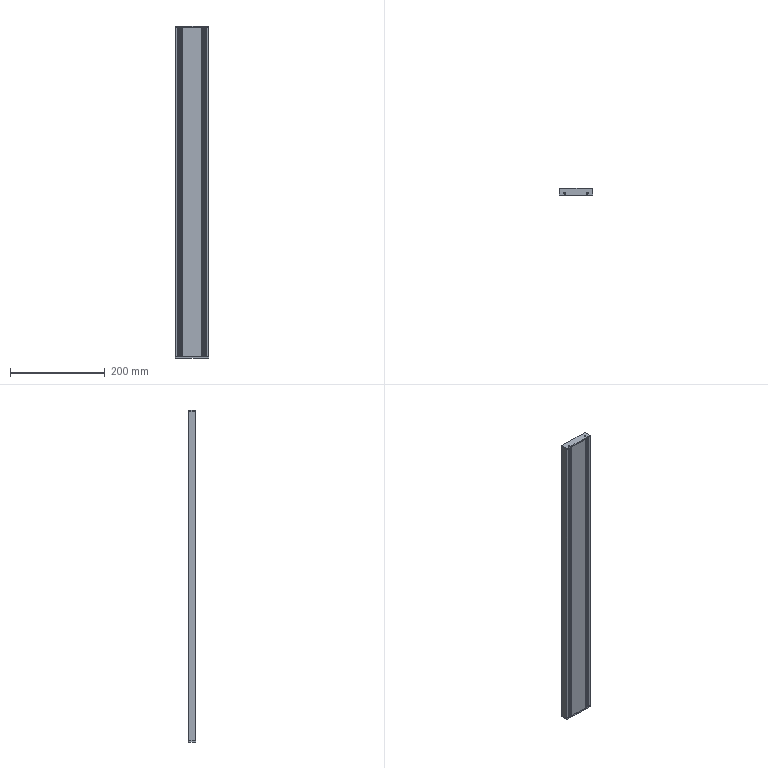Part | 4 solids | 926 faces | box 70 x 15 x 700 mm | volume 443111 mm3 | plane 877 | cylinder 49 | commonest cylinder face diameters 1 x12 2 x12 4 x8 6 x6 0.4 x4 1.1 x4